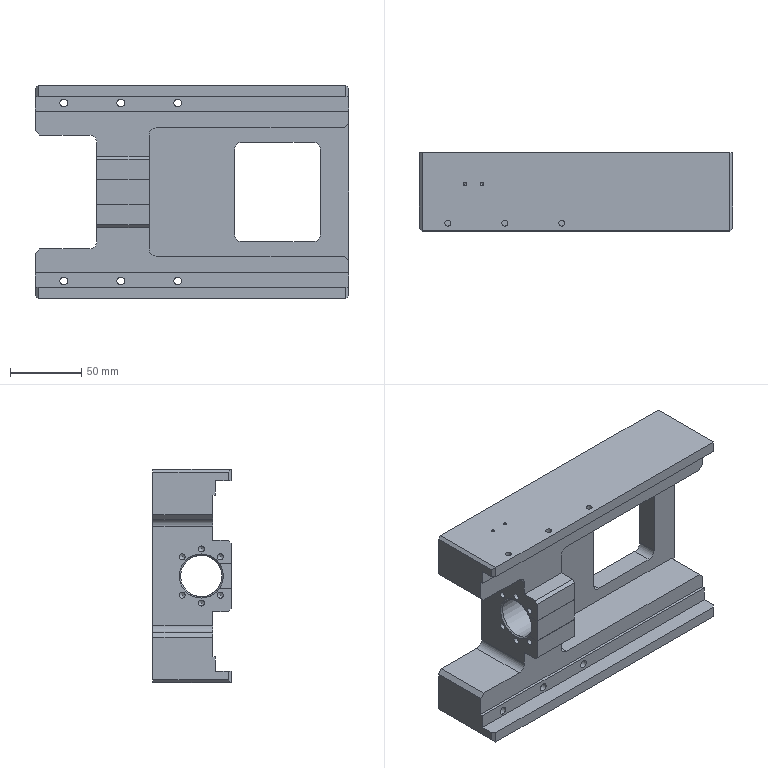Part | 2 solids | 237 faces | box 220 x 55 x 150 mm | volume 1723937 mm3 | plane 105 | cylinder 88 | cone 44 | commonest cylinder face diameters 10 x28 5 x20 4.2 x18 5.5 x12 2.5 x4 6 x4